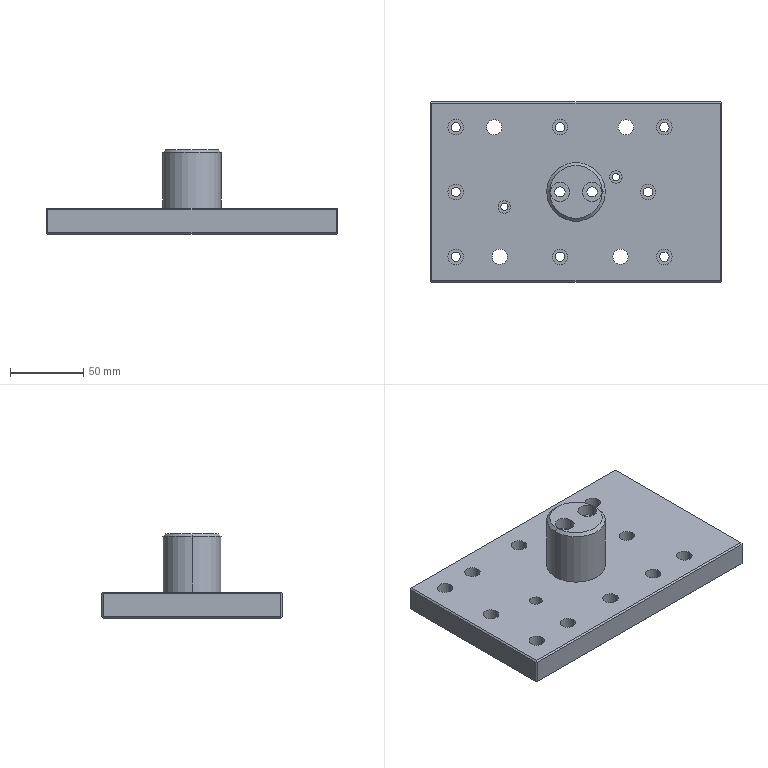Part | Creo | features CURVE 4, DATUM PLANE 3, CHAMFER 2, CUT 2, PROTRUSION 2, COORDINATE SYSTEM 1 | 1 solid | 91 faces | box 199.25 x 123.5 x 58 mm | volume 470509 mm3 | cylinder 58 | plane 31 | cone 2 | commonest cylinder face diameters 6.375 x16 10.658 x16 10.5 x8 5 x4 7 x4 8.5 x4